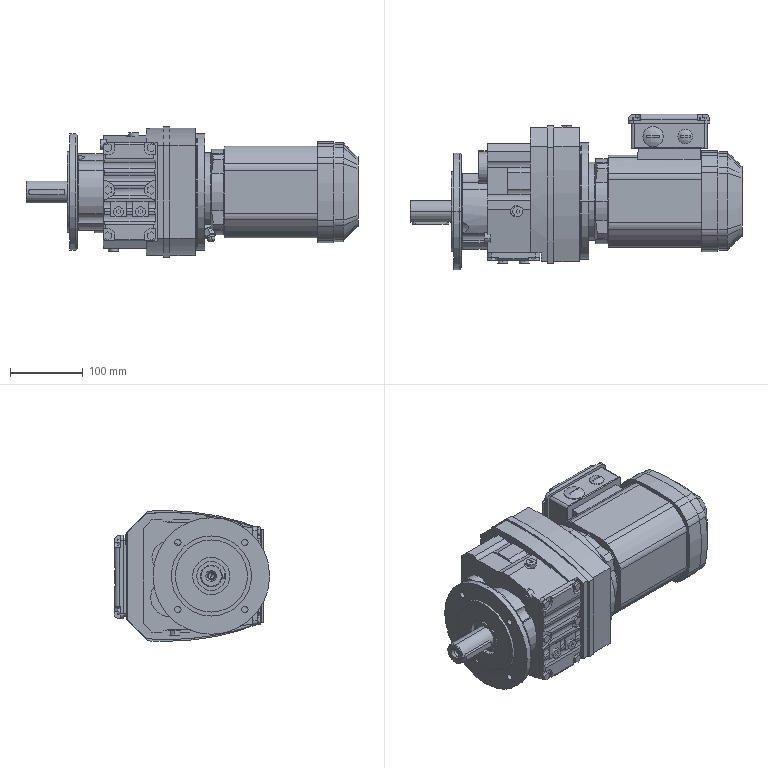Part | STEP file | PN_0044_geared motor | 20 solids | 738 faces | box 455.5 x 213.006 x 179.615 mm | volume 7890583 mm3 | plane 384 | cylinder 289 | cone 33 | spline 16 | torus 12 | sphere 2 | other 2 | commonest cylinder face diameters 0.1 x31 14 x24 40 x20 22 x19 9 x16 8 x14